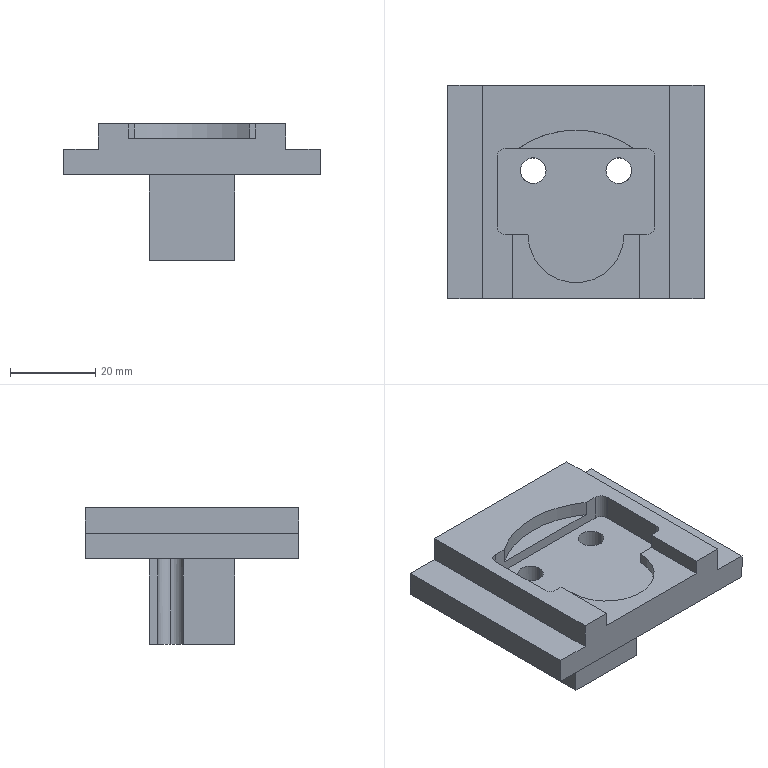Part | SolidWorks | features Cut 4, ICE 4, Extrusion 1, Fillet 1, MirrorPattern 1 | 1 solid | 37 faces | box 60 x 50 x 32 mm | volume 31490 mm3 | plane 27 | cylinder 10 | commonest cylinder face diameters 4 x4 6 x4 22.5 x1 47 x1
STEP:
#1=CARTESIAN_POINT('',(-7.,5.,6.));
#2=VERTEX_POINT('',#1);
#3=CARTESIAN_POINT('',(-13.,5.,6.));
#4=VERTEX_POINT('',#3);
#5=CARTESIAN_POINT('',(-10.,5.,6.));
#6=DIRECTION('',(0.,0.,-1.));
#7=DIRECTION('',(1.,0.,0.));
#8=AXIS2_PLACEMENT_3D('',#5,#6,#7);
#9=CIRCLE('',#8,3.);
#10=EDGE_CURVE('',#2,#4,#9,.T.);
#11=ORIENTED_EDGE('',*,*,#10,.F.);
#12=CARTESIAN_POINT('',(-7.,5.,-20.));
#13=VERTEX_POINT('',#12);
#14=CARTESIAN_POINT('',(-7.,5.,12.));
#15=DIRECTION('',(0.,0.,-1.));
#16=VECTOR('',#15,1000.);
#17=LINE('',#14,#16);
#18=EDGE_CURVE('',#2,#13,#17,.T.);
#19=ORIENTED_EDGE('',*,*,#18,.T.);
#20=CARTESIAN_POINT('',(-10.,2.,-20.));
#21=VERTEX_POINT('',#20);
#22=CARTESIAN_POINT('',(-10.,5.,-20.));
#23=DIRECTION('',(0.,0.,1.));
#24=DIRECTION('',(-1.,0.,0.));
#25=AXIS2_PLACEMENT_3D('',#22,#23,#24);
#26=CIRCLE('',#25,3.);
#27=EDGE_CURVE('',#21,#13,#26,.T.);
#28=ORIENTED_EDGE('',*,*,#27,.F.);
#29=CARTESIAN_POINT('',(-10.,2.,0.));
#30=VERTEX_POINT('',#29);
#31=CARTESIAN_POINT('',(-10.,2.,-20.001));
#32=DIRECTION('',(0.,0.,1.));
#33=VECTOR('',#32,1000.);
#34=LINE('',#31,#33);
#35=EDGE_CURVE('',#21,#30,#34,.T.);
#36=ORIENTED_EDGE('',*,*,#35,.T.);
#37=CARTESIAN_POINT('',(-13.,5.,0.));
#38=VERTEX_POINT('',#37);
#39=CARTESIAN_POINT('',(-10.,5.,0.));
#40=DIRECTION('',(0.,0.,-1.));
#41=DIRECTION('',(1.,0.,0.));
#42=AXIS2_PLACEMENT_3D('',#39,#40,#41);
#43=CIRCLE('',#42,3.);
#44=EDGE_CURVE('',#30,#38,#43,.T.);
#45=ORIENTED_EDGE('',*,*,#44,.T.);
#46=CARTESIAN_POINT('',(-13.,5.,12.));
#47=DIRECTION('',(0.,0.,-1.));
#48=VECTOR('',#47,1000.);
#49=LINE('',#46,#48);
#50=EDGE_CURVE('',#4,#38,#49,.T.);
#51=ORIENTED_EDGE('',*,*,#50,.F.);
#52=EDGE_LOOP('',(#11,#19,#28,#36,#45,#51));
#53=FACE_OUTER_BOUND('',#52,.T.);
#54=CARTESIAN_POINT('',(-10.,5.,12.));
#55=DIRECTION('',(0.,0.,-1.));
#56=DIRECTION('',(-1.,0.,0.));
#57=AXIS2_PLACEMENT_3D('',#54,#55,#56);
#58=CYLINDRICAL_SURFACE('',#57,3.);
#59=ADVANCED_FACE('',(#53),#58,.F.);
#60=CARTESIAN_POINT('',(13.,5.,6.));
#61=VERTEX_POINT('',#60);
#62=CARTESIAN_POINT('',(7.,5.,6.));
#63=VERTEX_POINT('',#62);
#64=CARTESIAN_POINT('',(10.,5.,6.));
#65=DIRECTION('',(0.,0.,-1.));
#66=DIRECTION('',(1.,0.,0.));
#67=AXIS2_PLACEMENT_3D('',#64,#65,#66);
#68=CIRCLE('',#67,3.);
#69=EDGE_CURVE('',#61,#63,#68,.T.);
#70=ORIENTED_EDGE('',*,*,#69,.F.);
#71=CARTESIAN_POINT('',(13.,5.,0.));
#72=VERTEX_POINT('',#71);
#73=CARTESIAN_POINT('',(13.,5.,12.));
#74=DIRECTION('',(0.,0.,-1.));
#75=VECTOR('',#74,1000.);
#76=LINE('',#73,#75);
#77=EDGE_CURVE('',#61,#72,#76,.T.);
#78=ORIENTED_EDGE('',*,*,#77,.T.);
#79=CARTESIAN_POINT('',(10.,2.,0.));
#80=VERTEX_POINT('',#79);
#81=CARTESIAN_POINT('',(10.,5.,0.));
#82=DIRECTION('',(0.,0.,-1.));
#83=DIRECTION('',(1.,0.,0.));
#84=AXIS2_PLACEMENT_3D('',#81,#82,#83);
#85=CIRCLE('',#84,3.);
#86=EDGE_CURVE('',#72,#80,#85,.T.);
#87=ORIENTED_EDGE('',*,*,#86,.T.);
#88=CARTESIAN_POINT('',(10.,2.,-20.));
#89=VERTEX_POINT('',#88);
#90=CARTESIAN_POINT('',(10.,2.,-20.001));
#91=DIRECTION('',(0.,0.,-1.));
#92=VECTOR('',#91,1000.);
#93=LINE('',#90,#92);
#94=EDGE_CURVE('',#80,#89,#93,.T.);
#95=ORIENTED_EDGE('',*,*,#94,.T.);
#96=CARTESIAN_POINT('',(7.,5.,-20.));
#97=VERTEX_POINT('',#96);
#98=CARTESIAN_POINT('',(10.,5.,-20.));
#99=DIRECTION('',(0.,0.,1.));
#100=DIRECTION('',(-1.,0.,0.));
#101=AXIS2_PLACEMENT_3D('',#98,#99,#100);
#102=CIRCLE('',#101,3.);
#103=EDGE_CURVE('',#97,#89,#102,.T.);
#104=ORIENTED_EDGE('',*,*,#103,.F.);
#105=CARTESIAN_POINT('',(7.,5.,12.));
#106=DIRECTION('',(0.,0.,-1.));
#107=VECTOR('',#106,1000.);
#108=LINE('',#105,#107);
#109=EDGE_CURVE('',#63,#97,#108,.T.);
#110=ORIENTED_EDGE('',*,*,#109,.F.);
#111=EDGE_LOOP('',(#70,#78,#87,#95,#104,#110));
#112=FACE_OUTER_BOUND('',#111,.T.);
#113=CARTESIAN_POINT('',(10.,5.,12.));
#114=DIRECTION('',(0.,0.,-1.));
#115=DIRECTION('',(-1.,0.,0.));
#116=AXIS2_PLACEMENT_3D('',#113,#114,#115);
#117=CYLINDRICAL_SURFACE('',#116,3.);
#118=ADVANCED_FACE('',(#112),#117,.F.);
#119=ORIENTED_EDGE('',*,*,#77,.F.);
#120=CARTESIAN_POINT('',(10.,5.,6.));
#121=DIRECTION('',(0.,0.,-1.));
#122=DIRECTION('',(1.,0.,0.));
#123=AXIS2_PLACEMENT_3D('',#120,#121,#122);
#124=CIRCLE('',#123,3.);
#125=EDGE_CURVE('',#63,#61,#124,.T.);
#126=ORIENTED_EDGE('',*,*,#125,.F.);
#127=ORIENTED_EDGE('',*,*,#109,.T.);
#128=CARTESIAN_POINT('',(10.,8.,-20.));
#129=VERTEX_POINT('',#128);
#130=CARTESIAN_POINT('',(10.,5.,-20.));
#131=DIRECTION('',(0.,0.,1.));
#132=DIRECTION('',(-1.,0.,0.));
#133=AXIS2_PLACEMENT_3D('',#130,#131,#132);
#134=CIRCLE('',#133,3.);
#135=EDGE_CURVE('',#129,#97,#134,.T.);
#136=ORIENTED_EDGE('',*,*,#135,.F.);
#137=CARTESIAN_POINT('',(10.,8.,0.));
#138=VERTEX_POINT('',#137);
#139=CARTESIAN_POINT('',(10.,8.,-20.001));
#140=DIRECTION('',(0.,0.,1.));
#141=VECTOR('',#140,1000.);
#142=LINE('',#139,#141);
#143=EDGE_CURVE('',#129,#138,#142,.T.);
#144=ORIENTED_EDGE('',*,*,#143,.T.);
#145=CARTESIAN_POINT('',(10.,5.,0.));
#146=DIRECTION('',(0.,0.,-1.));
#147=DIRECTION('',(1.,0.,0.));
#148=AXIS2_PLACEMENT_3D('',#145,#146,#147);
#149=CIRCLE('',#148,3.);
#150=EDGE_CURVE('',#138,#72,#149,.T.);
#151=ORIENTED_EDGE('',*,*,#150,.T.);
#152=EDGE_LOOP('',(#119,#126,#127,#136,#144,#151));
#153=FACE_OUTER_BOUND('',#152,.T.);
#154=CARTESIAN_POINT('',(10.,5.,12.));
#155=DIRECTION('',(0.,0.,-1.));
#156=DIRECTION('',(-1.,0.,0.));
#157=AXIS2_PLACEMENT_3D('',#154,#155,#156);
#158=CYLINDRICAL_SURFACE('',#157,3.);
#159=ADVANCED_FACE('',(#153),#158,.F.);
#160=CARTESIAN_POINT('',(11.25,-10.,8.5));
#161=VERTEX_POINT('',#160);
#162=CARTESIAN_POINT('',(14.923,-10.,8.5));
#163=VERTEX_POINT('',#162);
#164=CARTESIAN_POINT('',(17.,-10.,8.5));
#165=DIRECTION('',(1.,0.,0.));
#166=VECTOR('',#165,1000.);
#167=LINE('',#164,#166);
#168=EDGE_CURVE('',#161,#163,#167,.T.);
#169=ORIENTED_EDGE('',*,*,#168,.F.);
#170=CARTESIAN_POINT('',(-11.25,-10.,8.5));
#171=VERTEX_POINT('',#170);
#172=CARTESIAN_POINT('',(0.,-10.,8.5));
#173=DIRECTION('',(0.,0.,1.));
#174=DIRECTION('',(1.,0.,0.));
#175=AXIS2_PLACEMENT_3D('',#172,#173,#174);
#176=CIRCLE('',#175,11.25);
#177=EDGE_CURVE('',#171,#161,#176,.T.);
#178=ORIENTED_EDGE('',*,*,#177,.F.);
#179=CARTESIAN_POINT('',(-14.923,-10.,8.5));
#180=VERTEX_POINT('',#179);
#181=CARTESIAN_POINT('',(17.,-10.,8.5));
#182=DIRECTION('',(-1.,0.,0.));
#183=VECTOR('',#182,1000.);
#184=LINE('',#181,#183);
#185=EDGE_CURVE('',#171,#180,#184,.T.);
#186=ORIENTED_EDGE('',*,*,#185,.T.);
#187=CARTESIAN_POINT('',(-14.923,-25.,8.5));
#188=VERTEX_POINT('',#187);
#189=CARTESIAN_POINT('',(-14.923,0.,8.5));
#190=DIRECTION('',(0.,-1.,0.));
#191=VECTOR('',#190,1000.);
#192=LINE('',#189,#191);
#193=EDGE_CURVE('',#180,#188,#192,.T.);
#194=ORIENTED_EDGE('',*,*,#193,.T.);
#195=CARTESIAN_POINT('',(14.923,-25.,8.5));
#196=VERTEX_POINT('',#195);
#197=CARTESIAN_POINT('',(0.,-25.,8.5));
#198=DIRECTION('',(1.,0.,0.));
#199=VECTOR('',#198,1000.);
#200=LINE('',#197,#199);
#201=EDGE_CURVE('',#188,#196,#200,.T.);
#202=ORIENTED_EDGE('',*,*,#201,.T.);
#203=CARTESIAN_POINT('',(14.923,0.,8.5));
#204=DIRECTION('',(0.,-1.,0.));
#205=VECTOR('',#204,1000.);
#206=LINE('',#203,#205);
#207=EDGE_CURVE('',#163,#196,#206,.T.);
#208=ORIENTED_EDGE('',*,*,#207,.F.);
#209=EDGE_LOOP('',(#169,#178,#186,#194,#202,#208));
#210=FACE_OUTER_BOUND('',#209,.T.);
#211=CARTESIAN_POINT('',(17.,4.964,8.5));
#212=DIRECTION('',(0.,0.,1.));
#213=DIRECTION('',(1.,0.,0.));
#214=AXIS2_PLACEMENT_3D('',#211,#212,#213);
#215=PLANE('',#214);
#216=ADVANCED_FACE('',(#210),#215,.T.);
#217=CARTESIAN_POINT('',(14.923,-10.,12.));
#218=VERTEX_POINT('',#217);
#219=CARTESIAN_POINT('',(16.5,-10.,12.));
#220=VERTEX_POINT('',#219);
#221=CARTESIAN_POINT('',(0.,-10.,12.));
#222=DIRECTION('',(1.,0.,0.));
#223=VECTOR('',#222,1000.);
#224=LINE('',#221,#223);
#225=EDGE_CURVE('',#218,#220,#224,.T.);
#226=ORIENTED_EDGE('',*,*,#225,.F.);
#227=CARTESIAN_POINT('',(14.923,-25.,12.));
#228=VERTEX_POINT('',#227);
#229=CARTESIAN_POINT('',(14.923,0.,12.));
#230=DIRECTION('',(0.,-1.,0.));
#231=VECTOR('',#230,1000.);
#232=LINE('',#229,#231);
#233=EDGE_CURVE('',#218,#228,#232,.T.);
#234=ORIENTED_EDGE('',*,*,#233,.T.);
#235=CARTESIAN_POINT('',(22.,-25.,12.));
#236=VERTEX_POINT('',#235);
#237=CARTESIAN_POINT('',(30.,-25.,12.));
#238=DIRECTION('',(1.,0.,0.));
#239=VECTOR('',#238,1000.);
#240=LINE('',#237,#239);
#241=EDGE_CURVE('',#228,#236,#240,.T.);
#242=ORIENTED_EDGE('',*,*,#241,.T.);
#243=CARTESIAN_POINT('',(22.,25.,12.));
#244=VERTEX_POINT('',#243);
#245=CARTESIAN_POINT('',(22.,-25.,12.));
#246=DIRECTION('',(0.,-1.,0.));
#247=VECTOR('',#246,1000.);
#248=LINE('',#245,#247);
#249=EDGE_CURVE('',#244,#236,#248,.T.);
#250=ORIENTED_EDGE('',*,*,#249,.F.);
#251=CARTESIAN_POINT('',(-22.,25.,12.));
#252=VERTEX_POINT('',#251);
#253=CARTESIAN_POINT('',(30.,25.,12.));
#254=DIRECTION('',(-1.,0.,0.));
#255=VECTOR('',#254,1000.);
#256=LINE('',#253,#255);
#257=EDGE_CURVE('',#244,#252,#256,.T.);
#258=ORIENTED_EDGE('',*,*,#257,.T.);
#259=CARTESIAN_POINT('',(-22.,-25.,12.));
#260=VERTEX_POINT('',#259);
#261=CARTESIAN_POINT('',(-22.,25.,12.));
#262=DIRECTION('',(0.,1.,0.));
#263=VECTOR('',#262,1000.);
#264=LINE('',#261,#263);
#265=EDGE_CURVE('',#260,#252,#264,.T.);
#266=ORIENTED_EDGE('',*,*,#265,.F.);
#267=CARTESIAN_POINT('',(-14.923,-25.,12.));
#268=VERTEX_POINT('',#267);
#269=CARTESIAN_POINT('',(30.,-25.,12.));
#270=DIRECTION('',(1.,0.,0.));
#271=VECTOR('',#270,1000.);
#272=LINE('',#269,#271);
#273=EDGE_CURVE('',#260,#268,#272,.T.);
#274=ORIENTED_EDGE('',*,*,#273,.T.);
#275=CARTESIAN_POINT('',(-14.923,-10.,12.));
#276=VERTEX_POINT('',#275);
#277=CARTESIAN_POINT('',(-14.923,0.,12.));
#278=DIRECTION('',(0.,-1.,0.));
#279=VECTOR('',#278,1000.);
#280=LINE('',#277,#279);
#281=EDGE_CURVE('',#276,#268,#280,.T.);
#282=ORIENTED_EDGE('',*,*,#281,.F.);
#283=CARTESIAN_POINT('',(-16.5,-10.,12.));
#284=VERTEX_POINT('',#283);
#285=CARTESIAN_POINT('',(0.,-10.,12.));
#286=DIRECTION('',(-1.,0.,0.));
#287=VECTOR('',#286,1000.);
#288=LINE('',#285,#287);
#289=EDGE_CURVE('',#276,#284,#288,.T.);
#290=ORIENTED_EDGE('',*,*,#289,.T.);
#291=CARTESIAN_POINT('',(-18.5,-8.,12.));
#292=VERTEX_POINT('',#291);
#293=CARTESIAN_POINT('',(-16.5,-8.,12.));
#294=DIRECTION('',(0.,0.,-1.));
#295=DIRECTION('',(1.,0.,0.));
#296=AXIS2_PLACEMENT_3D('',#293,#294,#295);
#297=CIRCLE('',#296,2.);
#298=EDGE_CURVE('',#284,#292,#297,.T.);
#299=ORIENTED_EDGE('',*,*,#298,.T.);
#300=CARTESIAN_POINT('',(-18.5,8.2,12.));
#301=VERTEX_POINT('',#300);
#302=CARTESIAN_POINT('',(-18.5,4.964,12.));
#303=DIRECTION('',(0.,-1.,0.));
#304=VECTOR('',#303,1000.);
#305=LINE('',#302,#304);
#306=EDGE_CURVE('',#301,#292,#305,.T.);
#307=ORIENTED_EDGE('',*,*,#306,.F.);
#308=CARTESIAN_POINT('',(-16.5,10.2,12.));
#309=VERTEX_POINT('',#308);
#310=CARTESIAN_POINT('',(-16.5,8.2,12.));
#311=DIRECTION('',(0.,0.,-1.));
#312=DIRECTION('',(1.,0.,0.));
#313=AXIS2_PLACEMENT_3D('',#310,#311,#312);
#314=CIRCLE('',#313,2.);
#315=EDGE_CURVE('',#301,#309,#314,.T.);
#316=ORIENTED_EDGE('',*,*,#315,.T.);
#317=CARTESIAN_POINT('',(-13.55,10.2,12.));
#318=VERTEX_POINT('',#317);
#319=CARTESIAN_POINT('',(0.,10.2,12.));
#320=DIRECTION('',(1.,0.,0.));
#321=VECTOR('',#320,1000.);
#322=LINE('',#319,#321);
#323=EDGE_CURVE('',#309,#318,#322,.T.);
#324=ORIENTED_EDGE('',*,*,#323,.T.);
#325=CARTESIAN_POINT('',(13.55,10.2,12.));
#326=VERTEX_POINT('',#325);
#327=CARTESIAN_POINT('',(0.,-9.,12.));
#328=DIRECTION('',(0.,0.,1.));
#329=DIRECTION('',(1.,0.,0.));
#330=AXIS2_PLACEMENT_3D('',#327,#328,#329);
#331=CIRCLE('',#330,23.5);
#332=EDGE_CURVE('',#326,#318,#331,.T.);
#333=ORIENTED_EDGE('',*,*,#332,.F.);
#334=CARTESIAN_POINT('',(16.5,10.2,12.));
#335=VERTEX_POINT('',#334);
#336=CARTESIAN_POINT('',(0.,10.2,12.));
#337=DIRECTION('',(-1.,0.,0.));
#338=VECTOR('',#337,1000.);
#339=LINE('',#336,#338);
#340=EDGE_CURVE('',#335,#326,#339,.T.);
#341=ORIENTED_EDGE('',*,*,#340,.F.);
#342=CARTESIAN_POINT('',(18.5,8.2,12.));
#343=VERTEX_POINT('',#342);
#344=CARTESIAN_POINT('',(16.5,8.2,12.));
#345=DIRECTION('',(0.,0.,-1.));
#346=DIRECTION('',(1.,0.,0.));
#347=AXIS2_PLACEMENT_3D('',#344,#345,#346);
#348=CIRCLE('',#347,2.);
#349=EDGE_CURVE('',#335,#343,#348,.T.);
#350=ORIENTED_EDGE('',*,*,#349,.T.);
#351=CARTESIAN_POINT('',(18.5,-8.,12.));
#352=VERTEX_POINT('',#351);
#353=CARTESIAN_POINT('',(18.5,-1.5,12.));
#354=DIRECTION('',(0.,1.,0.));
#355=VECTOR('',#354,1000.);
#356=LINE('',#353,#355);
#357=EDGE_CURVE('',#352,#343,#356,.T.);
#358=ORIENTED_EDGE('',*,*,#357,.F.);
#359=CARTESIAN_POINT('',(16.5,-8.,12.));
#360=DIRECTION('',(0.,0.,-1.));
#361=DIRECTION('',(1.,0.,0.));
#362=AXIS2_PLACEMENT_3D('',#359,#360,#361);
#363=CIRCLE('',#362,2.);
#364=EDGE_CURVE('',#352,#220,#363,.T.);
#365=ORIENTED_EDGE('',*,*,#364,.T.);
#366=EDGE_LOOP('',(#226,#234,#242,#250,#258,#266,#274,#282,#290,#299,#307,#316,#324,#333,#341,#350,#358,#365));
#367=FACE_OUTER_BOUND('',#366,.T.);
#368=CARTESIAN_POINT('',(0.,0.,12.));
#369=DIRECTION('',(0.,0.,1.));
#370=DIRECTION('',(1.,0.,0.));
#371=AXIS2_PLACEMENT_3D('',#368,#369,#370);
#372=PLANE('',#371);
#373=ADVANCED_FACE('',(#367),#372,.T.);
#374=CARTESIAN_POINT('',(13.55,10.2,8.5));
#375=VERTEX_POINT('',#374);
#376=CARTESIAN_POINT('',(-13.55,10.2,8.5));
#377=VERTEX_POINT('',#376);
#378=CARTESIAN_POINT('',(0.,-9.,8.5));
#379=DIRECTION('',(0.,0.,1.));
#380=DIRECTION('',(1.,0.,0.));
#381=AXIS2_PLACEMENT_3D('',#378,#379,#380);
#382=CIRCLE('',#381,23.5);
#383=EDGE_CURVE('',#375,#377,#382,.T.);
#384=ORIENTED_EDGE('',*,*,#383,.F.);
#385=CARTESIAN_POINT('',(13.55,10.2,8.5));
#386=DIRECTION('',(0.,0.,1.));
#387=VECTOR('',#386,1000.);
#388=LINE('',#385,#387);
#389=EDGE_CURVE('',#375,#326,#388,.T.);
#390=ORIENTED_EDGE('',*,*,#389,.T.);
#391=ORIENTED_EDGE('',*,*,#332,.T.);
#392=CARTESIAN_POINT('',(-13.55,10.2,8.5));
#393=DIRECTION('',(0.,0.,1.));
#394=VECTOR('',#393,1000.);
#395=LINE('',#392,#394);
#396=EDGE_CURVE('',#377,#318,#395,.T.);
#397=ORIENTED_EDGE('',*,*,#396,.F.);
#398=EDGE_LOOP('',(#384,#390,#391,#397));
#399=FACE_OUTER_BOUND('',#398,.T.);
#400=CARTESIAN_POINT('',(0.,-9.,8.5));
#401=DIRECTION('',(0.,0.,1.));
#402=DIRECTION('',(1.,0.,0.));
#403=AXIS2_PLACEMENT_3D('',#400,#401,#402);
#404=CYLINDRICAL_SURFACE('',#403,23.5);
#405=ADVANCED_FACE('',(#399),#404,.F.);
#406=CARTESIAN_POINT('',(3.937,10.2,8.5));
#407=DIRECTION('',(-1.,0.,0.));
#408=VECTOR('',#407,1000.);
#409=LINE('',#406,#408);
#410=EDGE_CURVE('',#375,#377,#409,.T.);
#411=ORIENTED_EDGE('',*,*,#410,.F.);
#412=ORIENTED_EDGE('',*,*,#383,.T.);
#413=EDGE_LOOP('',(#411,#412));
#414=FACE_OUTER_BOUND('',#413,.T.);
#415=CARTESIAN_POINT('',(17.,4.964,8.5));
#416=DIRECTION('',(0.,0.,1.));
#417=DIRECTION('',(1.,0.,0.));
#418=AXIS2_PLACEMENT_3D('',#415,#416,#417);
#419=PLANE('',#418);
#420=ADVANCED_FACE('',(#414),#419,.T.);
#421=CARTESIAN_POINT('',(-14.923,-10.,8.5));
#422=DIRECTION('',(0.,0.,-1.));
#423=VECTOR('',#422,1000.);
#424=LINE('',#421,#423);
#425=EDGE_CURVE('',#276,#180,#424,.T.);
#426=ORIENTED_EDGE('',*,*,#425,.F.);
#427=ORIENTED_EDGE('',*,*,#281,.T.);
#428=CARTESIAN_POINT('',(-14.923,-25.,8.5));
#429=DIRECTION('',(0.,0.,1.));
#430=VECTOR('',#429,1000.);
#431=LINE('',#428,#430);
#432=EDGE_CURVE('',#188,#268,#431,.T.);
#433=ORIENTED_EDGE('',*,*,#432,.F.);
#434=ORIENTED_EDGE('',*,*,#193,.F.);
#435=EDGE_LOOP('',(#426,#427,#433,#434));
#436=FACE_OUTER_BOUND('',#435,.T.);
#437=CARTESIAN_POINT('',(-14.923,0.,8.5));
#438=DIRECTION('',(-1.,0.,0.));
#439=DIRECTION('',(0.,0.,1.));
#440=AXIS2_PLACEMENT_3D('',#437,#438,#439);
#441=PLANE('',#440);
#442=ADVANCED_FACE('',(#436),#441,.F.);
#443=ORIENTED_EDGE('',*,*,#177,.T.);
#444=CARTESIAN_POINT('',(11.25,-10.,6.));
#445=VERTEX_POINT('',#444);
#446=CARTESIAN_POINT('',(11.25,-10.,6.));
#447=DIRECTION('',(0.,0.,-1.));
#448=VECTOR('',#447,1000.);
#449=LINE('',#446,#448);
#450=EDGE_CURVE('',#161,#445,#449,.T.);
#451=ORIENTED_EDGE('',*,*,#450,.T.);
#452=CARTESIAN_POINT('',(-11.25,-10.,6.));
#453=VERTEX_POINT('',#452);
#454=CARTESIAN_POINT('',(0.,-10.,6.));
#455=DIRECTION('',(0.,0.,1.));
#456=DIRECTION('',(1.,0.,0.));
#457=AXIS2_PLACEMENT_3D('',#454,#455,#456);
#458=CIRCLE('',#457,11.25);
#459=EDGE_CURVE('',#453,#445,#458,.T.);
#460=ORIENTED_EDGE('',*,*,#459,.F.);
#461=CARTESIAN_POINT('',(-11.25,-10.,6.));
#462=DIRECTION('',(0.,0.,-1.));
#463=VECTOR('',#462,1000.);
#464=LINE('',#461,#463);
#465=EDGE_CURVE('',#171,#453,#464,.T.);
#466=ORIENTED_EDGE('',*,*,#465,.F.);
#467=EDGE_LOOP('',(#443,#451,#460,#466));
#468=FACE_OUTER_BOUND('',#467,.T.);
#469=CARTESIAN_POINT('',(0.,-10.,6.));
#470=DIRECTION('',(0.,0.,1.));
#471=DIRECTION('',(1.,0.,0.));
#472=AXIS2_PLACEMENT_3D('',#469,#470,#471);
#473=CYLINDRICAL_SURFACE('',#472,11.25);
#474=ADVANCED_FACE('',(#468),#473,.F.);
#475=ORIENTED_EDGE('',*,*,#18,.F.);
#476=CARTESIAN_POINT('',(-10.,5.,6.));
#477=DIRECTION('',(0.,0.,-1.));
#478=DIRECTION('',(1.,0.,0.));
#479=AXIS2_PLACEMENT_3D('',#476,#477,#478);
#480=CIRCLE('',#479,3.);
#481=EDGE_CURVE('',#4,#2,#480,.T.);
#482=ORIENTED_EDGE('',*,*,#481,.F.);
#483=ORIENTED_EDGE('',*,*,#50,.T.);
#484=CARTESIAN_POINT('',(-10.,8.,0.));
#485=VERTEX_POINT('',#484);
#486=CARTESIAN_POINT('',(-10.,5.,0.));
#487=DIRECTION('',(0.,0.,-1.));
#488=DIRECTION('',(1.,0.,0.));
#489=AXIS2_PLACEMENT_3D('',#486,#487,#488);
#490=CIRCLE('',#489,3.);
#491=EDGE_CURVE('',#38,#485,#490,.T.);
#492=ORIENTED_EDGE('',*,*,#491,.T.);
#493=CARTESIAN_POINT('',(-10.,8.,-20.));
#494=VERTEX_POINT('',#493);
#495=CARTESIAN_POINT('',(-10.,8.,-20.001));
#496=DIRECTION('',(0.,0.,-1.));
#497=VECTOR('',#496,1000.);
#498=LINE('',#495,#497);
#499=EDGE_CURVE('',#485,#494,#498,.T.);
#500=ORIENTED_EDGE('',*,*,#499,.T.);
#501=CARTESIAN_POINT('',(-10.,5.,-20.));
#502=DIRECTION('',(0.,0.,1.));
#503=DIRECTION('',(-1.,0.,0.));
#504=AXIS2_PLACEMENT_3D('',#501,#502,#503);
#505=CIRCLE('',#504,3.);
#506=EDGE_CURVE('',#13,#494,#505,.T.);
#507=ORIENTED_EDGE('',*,*,#506,.F.);
#508=EDGE_LOOP('',(#475,#482,#483,#492,#500,#507));
#509=FACE_OUTER_BOUND('',#508,.T.);
#510=CARTESIAN_POINT('',(-10.,5.,12.));
#511=DIRECTION('',(0.,0.,-1.));
#512=DIRECTION('',(-1.,0.,0.));
#513=AXIS2_PLACEMENT_3D('',#510,#511,#512);
#514=CYLINDRICAL_SURFACE('',#513,3.);
#515=ADVANCED_FACE('',(#509),#514,.F.);
#516=CARTESIAN_POINT('',(-30.,25.,6.));
#517=VERTEX_POINT('',#516);
#518=CARTESIAN_POINT('',(-30.,-25.,6.));
#519=VERTEX_POINT('',#518);
#520=CARTESIAN_POINT('',(-30.,25.,6.));
#521=DIRECTION('',(0.,-1.,0.));
#522=VECTOR('',#521,1000.);
#523=LINE('',#520,#522);
#524=EDGE_CURVE('',#517,#519,#523,.T.);
#525=ORIENTED_EDGE('',*,*,#524,.F.);
#526=CARTESIAN_POINT('',(-30.,25.,0.));
#527=VERTEX_POINT('',#526);
#528=CARTESIAN_POINT('',(-30.,25.,12.));
#529=DIRECTION('',(0.,0.,-1.));
#530=VECTOR('',#529,1000.);
#531=LINE('',#528,#530);
#532=EDGE_CURVE('',#517,#527,#531,.T.);
#533=ORIENTED_EDGE('',*,*,#532,.T.);
#534=CARTESIAN_POINT('',(-30.,-25.,0.));
#535=VERTEX_POINT('',#534);
#536=CARTESIAN_POINT('',(-30.,-25.,0.));
#537=DIRECTION('',(0.,-1.,0.));
#538=VECTOR('',#537,1000.);
#539=LINE('',#536,#538);
#540=EDGE_CURVE('',#527,#535,#539,.T.);
#541=ORIENTED_EDGE('',*,*,#540,.T.);
#542=CARTESIAN_POINT('',(-30.,-25.,12.));
#543=DIRECTION('',(0.,0.,-1.));
#544=VECTOR('',#543,1000.);
#545=LINE('',#542,#544);
#546=EDGE_CURVE('',#519,#535,#545,.T.);
#547=ORIENTED_EDGE('',*,*,#546,.F.);
#548=EDGE_LOOP('',(#525,#533,#541,#547));
#549=FACE_OUTER_BOUND('',#548,.T.);
#550=CARTESIAN_POINT('',(-30.,-25.,12.));
#551=DIRECTION('',(1.,0.,0.));
#552=DIRECTION('',(0.,0.,-1.));
#553=AXIS2_PLACEMENT_3D('',#550,#551,#552);
#554=PLANE('',#553);
#555=ADVANCED_FACE('',(#549),#554,.F.);
#556=CARTESIAN_POINT('',(30.,-25.,6.));
#557=VERTEX_POINT('',#556);
#558=CARTESIAN_POINT('',(30.,25.,6.));
#559=VERTEX_POINT('',#558);
#560=CARTESIAN_POINT('',(30.,-25.,6.));
#561=DIRECTION('',(0.,1.,0.));
#562=VECTOR('',#561,1000.);
#563=LINE('',#560,#562);
#564=EDGE_CURVE('',#557,#559,#563,.T.);
#565=ORIENTED_EDGE('',*,*,#564,.F.);
#566=CARTESIAN_POINT('',(30.,-25.,0.));
#567=VERTEX_POINT('',#566);
#568=CARTESIAN_POINT('',(30.,-25.,12.));
#569=DIRECTION('',(0.,0.,-1.));
#570=VECTOR('',#569,1000.);
#571=LINE('',#568,#570);
#572=EDGE_CURVE('',#557,#567,#571,.T.);
#573=ORIENTED_EDGE('',*,*,#572,.T.);
#574=CARTESIAN_POINT('',(30.,25.,0.));
#575=VERTEX_POINT('',#574);
#576=CARTESIAN_POINT('',(30.,-25.,0.));
#577=DIRECTION('',(0.,1.,0.));
#578=VECTOR('',#577,1000.);
#579=LINE('',#576,#578);
#580=EDGE_CURVE('',#567,#575,#579,.T.);
#581=ORIENTED_EDGE('',*,*,#580,.T.);
#582=CARTESIAN_POINT('',(30.,25.,12.));
#583=DIRECTION('',(0.,0.,-1.));
#584=VECTOR('',#583,1000.);
#585=LINE('',#582,#584);
#586=EDGE_CURVE('',#559,#575,#585,.T.);
#587=ORIENTED_EDGE('',*,*,#586,.F.);
#588=EDGE_LOOP('',(#565,#573,#581,#587));
#589=FACE_OUTER_BOUND('',#588,.T.);
#590=CARTESIAN_POINT('',(30.,-25.,12.));
#591=DIRECTION('',(-1.,0.,0.));
#592=DIRECTION('',(0.,-1.,0.));
#593=AXIS2_PLACEMENT_3D('',#590,#591,#592);
#594=PLANE('',#593);
#595=ADVANCED_FACE('',(#589),#594,.F.);
#596=ORIENTED_EDGE('',*,*,#540,.F.);
#597=CARTESIAN_POINT('',(30.,25.,0.));
#598=DIRECTION('',(-1.,0.,0.));
#599=VECTOR('',#598,1000.);
#600=LINE('',#597,#599);
#601=EDGE_CURVE('',#575,#527,#600,.T.);
#602=ORIENTED_EDGE('',*,*,#601,.F.);
#603=ORIENTED_EDGE('',*,*,#580,.F.);
#604=CARTESIAN_POINT('',(30.,-25.,0.));
#605=DIRECTION('',(1.,0.,0.));
#606=VECTOR('',#605,1000.);
#607=LINE('',#604,#606);
#608=EDGE_CURVE('',#535,#567,#607,.T.);
#609=ORIENTED_EDGE('',*,*,#608,.F.);
#610=EDGE_LOOP('',(#596,#602,#603,#609));
#611=FACE_OUTER_BOUND('',#610,.T.);
#612=ORIENTED_EDGE('',*,*,#44,.F.);
#613=CARTESIAN_POINT('',(-10.,-10.,0.));
#614=VERTEX_POINT('',#613);
#615=CARTESIAN_POINT('',(-10.,-10.,0.));
#616=DIRECTION('',(0.,1.,0.));
#617=VECTOR('',#616,1000.);
#618=LINE('',#615,#617);
#619=EDGE_CURVE('',#614,#30,#618,.T.);
#620=ORIENTED_EDGE('',*,*,#619,.F.);
#621=CARTESIAN_POINT('',(10.,-10.,0.));
#622=VERTEX_POINT('',#621);
#623=CARTESIAN_POINT('',(-10.,-10.,0.));
#624=DIRECTION('',(-1.,0.,0.));
#625=VECTOR('',#624,1000.);
#626=LINE('',#623,#625);
#627=EDGE_CURVE('',#622,#614,#626,.T.);
#628=ORIENTED_EDGE('',*,*,#627,.F.);
#629=CARTESIAN_POINT('',(10.,-10.,0.));
#630=DIRECTION('',(0.,-1.,0.));
#631=VECTOR('',#630,1000.);
#632=LINE('',#629,#631);
#633=EDGE_CURVE('',#80,#622,#632,.T.);
#634=ORIENTED_EDGE('',*,*,#633,.F.);
#635=ORIENTED_EDGE('',*,*,#86,.F.);
#636=ORIENTED_EDGE('',*,*,#150,.F.);
#637=CARTESIAN_POINT('',(10.,10.,0.));
#638=VERTEX_POINT('',#637);
#639=CARTESIAN_POINT('',(10.,-10.,0.));
#640=DIRECTION('',(0.,-1.,0.));
#641=VECTOR('',#640,1000.);
#642=LINE('',#639,#641);
#643=EDGE_CURVE('',#638,#138,#642,.T.);
#644=ORIENTED_EDGE('',*,*,#643,.F.);
#645=CARTESIAN_POINT('',(-10.,10.,0.));
#646=VERTEX_POINT('',#645);
#647=CARTESIAN_POINT('',(-10.,10.,0.));
#648=DIRECTION('',(1.,0.,0.));
#649=VECTOR('',#648,1000.);
#650=LINE('',#647,#649);
#651=EDGE_CURVE('',#646,#638,#650,.T.);
#652=ORIENTED_EDGE('',*,*,#651,.F.);
#653=CARTESIAN_POINT('',(-10.,-10.,0.));
#654=DIRECTION('',(0.,1.,0.));
#655=VECTOR('',#654,1000.);
#656=LINE('',#653,#655);
#657=EDGE_CURVE('',#485,#646,#656,.T.);
#658=ORIENTED_EDGE('',*,*,#657,.F.);
#659=ORIENTED_EDGE('',*,*,#491,.F.);
#660=EDGE_LOOP('',(#612,#620,#628,#634,#635,#636,#644,#652,#658,#659));
#661=FACE_BOUND('',#660,.T.);
#662=CARTESIAN_POINT('',(0.,0.,0.));
#663=DIRECTION('',(0.,0.,1.));
#664=DIRECTION('',(1.,0.,0.));
#665=AXIS2_PLACEMENT_3D('',#662,#663,#664);
#666=PLANE('',#665);
#667=ADVANCED_FACE('',(#611,#661),#666,.F.);
#668=ORIENTED_EDGE('',*,*,#143,.F.);
#669=CARTESIAN_POINT('',(10.,10.,-20.));
#670=VERTEX_POINT('',#669);
#671=CARTESIAN_POINT('',(10.,-10.,-20.));
#672=DIRECTION('',(0.,-1.,0.));
#673=VECTOR('',#672,1000.);
#674=LINE('',#671,#673);
#675=EDGE_CURVE('',#670,#129,#674,.T.);
#676=ORIENTED_EDGE('',*,*,#675,.F.);
#677=CARTESIAN_POINT('',(10.,10.,-20.));
#678=DIRECTION('',(0.,0.,1.));
#679=VECTOR('',#678,1000.);
#680=LINE('',#677,#679);
#681=EDGE_CURVE('',#670,#638,#680,.T.);
#682=ORIENTED_EDGE('',*,*,#681,.T.);
#683=ORIENTED_EDGE('',*,*,#643,.T.);
#684=EDGE_LOOP('',(#668,#676,#682,#683));
#685=FACE_OUTER_BOUND('',#684,.T.);
#686=CARTESIAN_POINT('',(10.,-10.,-20.));
#687=DIRECTION('',(-1.,0.,0.));
#688=DIRECTION('',(0.,0.,1.));
#689=AXIS2_PLACEMENT_3D('',#686,#687,#688);
#690=PLANE('',#689);
#691=ADVANCED_FACE('',(#685),#690,.F.);
#692=ORIENTED_EDGE('',*,*,#94,.F.);
#693=ORIENTED_EDGE('',*,*,#633,.T.);
#694=CARTESIAN_POINT('',(10.,-10.,-20.));
#695=VERTEX_POINT('',#694);
#696=CARTESIAN_POINT('',(10.,-10.,-20.));
#697=DIRECTION('',(0.,0.,1.));
#698=VECTOR('',#697,1000.);
#699=LINE('',#696,#698);
#700=EDGE_CURVE('',#695,#622,#699,.T.);
#701=ORIENTED_EDGE('',*,*,#700,.F.);
#702=CARTESIAN_POINT('',(10.,-10.,-20.));
#703=DIRECTION('',(0.,-1.,0.));
#704=VECTOR('',#703,1000.);
#705=LINE('',#702,#704);
#706=EDGE_CURVE('',#89,#695,#705,.T.);
#707=ORIENTED_EDGE('',*,*,#706,.F.);
#708=EDGE_LOOP('',(#692,#693,#701,#707));
#709=FACE_OUTER_BOUND('',#708,.T.);
#710=CARTESIAN_POINT('',(10.,-10.,-20.));
#711=DIRECTION('',(-1.,0.,0.));
#712=DIRECTION('',(0.,0.,1.));
#713=AXIS2_PLACEMENT_3D('',#710,#711,#712);
#714=PLANE('',#713);
#715=ADVANCED_FACE('',(#709),#714,.F.);
#716=ORIENTED_EDGE('',*,*,#35,.F.);
#717=CARTESIAN_POINT('',(-10.,-10.,-20.));
#718=VERTEX_POINT('',#717);
#719=CARTESIAN_POINT('',(-10.,-10.,-20.));
#720=DIRECTION('',(0.,1.,0.));
#721=VECTOR('',#720,1000.);
#722=LINE('',#719,#721);
#723=EDGE_CURVE('',#718,#21,#722,.T.);
#724=ORIENTED_EDGE('',*,*,#723,.F.);
#725=CARTESIAN_POINT('',(-10.,-10.,-20.));
#726=DIRECTION('',(0.,0.,1.));
#727=VECTOR('',#726,1000.);
#728=LINE('',#725,#727);
#729=EDGE_CURVE('',#718,#614,#728,.T.);
#730=ORIENTED_EDGE('',*,*,#729,.T.);
#731=ORIENTED_EDGE('',*,*,#619,.T.);
#732=EDGE_LOOP('',(#716,#724,#730,#731));
#733=FACE_OUTER_BOUND('',#732,.T.);
#734=CARTESIAN_POINT('',(-10.,-10.,-20.));
#735=DIRECTION('',(1.,0.,0.));
#736=DIRECTION('',(0.,0.,-1.));
#737=AXIS2_PLACEMENT_3D('',#734,#735,#736);
#738=PLANE('',#737);
#739=ADVANCED_FACE('',(#733),#738,.F.);
#740=ORIENTED_EDGE('',*,*,#499,.F.);
#741=ORIENTED_EDGE('',*,*,#657,.T.);
#742=CARTESIAN_POINT('',(-10.,10.,-20.));
#743=VERTEX_POINT('',#742);
#744=CARTESIAN_POINT('',(-10.,10.,-20.));
#745=DIRECTION('',(0.,0.,1.));
#746=VECTOR('',#745,1000.);
#747=LINE('',#744,#746);
#748=EDGE_CURVE('',#743,#646,#747,.T.);
#749=ORIENTED_EDGE('',*,*,#748,.F.);
#750=CARTESIAN_POINT('',(-10.,-10.,-20.));
#751=DIRECTION('',(0.,1.,0.));
#752=VECTOR('',#751,1000.);
#753=LINE('',#750,#752);
#754=EDGE_CURVE('',#494,#743,#753,.T.);
#755=ORIENTED_EDGE('',*,*,#754,.F.);
#756=EDGE_LOOP('',(#740,#741,#749,#755));
#757=FACE_OUTER_BOUND('',#756,.T.);
#758=CARTESIAN_POINT('',(-10.,-10.,-20.));
#759=DIRECTION('',(1.,0.,0.));
#760=DIRECTION('',(0.,0.,-1.));
#761=AXIS2_PLACEMENT_3D('',#758,#759,#760);
#762=PLANE('',#761);
#763=ADVANCED_FACE('',(#757),#762,.F.);
#764=ORIENTED_EDGE('',*,*,#723,.T.);
#765=ORIENTED_EDGE('',*,*,#27,.T.);
#766=ORIENTED_EDGE('',*,*,#506,.T.);
#767=ORIENTED_EDGE('',*,*,#754,.T.);
#768=CARTESIAN_POINT('',(-10.,10.,-20.));
#769=DIRECTION('',(1.,0.,0.));
#770=VECTOR('',#769,1000.);
#771=LINE('',#768,#770);
#772=EDGE_CURVE('',#743,#670,#771,.T.);
#773=ORIENTED_EDGE('',*,*,#772,.T.);
#774=ORIENTED_EDGE('',*,*,#675,.T.);
#775=ORIENTED_EDGE('',*,*,#135,.T.);
#776=ORIENTED_EDGE('',*,*,#103,.T.);
#777=ORIENTED_EDGE('',*,*,#706,.T.);
#778=CARTESIAN_POINT('',(-10.,-10.,-20.));
#779=DIRECTION('',(-1.,0.,0.));
#780=VECTOR('',#779,1000.);
#781=LINE('',#778,#780);
#782=EDGE_CURVE('',#695,#718,#781,.T.);
#783=ORIENTED_EDGE('',*,*,#782,.T.);
#784=EDGE_LOOP('',(#764,#765,#766,#767,#773,#774,#775,#776,#777,#783));
#785=FACE_OUTER_BOUND('',#784,.T.);
#786=CARTESIAN_POINT('',(0.,0.,-20.));
#787=DIRECTION('',(0.,0.,-1.));
#788=DIRECTION('',(-1.,0.,0.));
#789=AXIS2_PLACEMENT_3D('',#786,#787,#788);
#790=PLANE('',#789);
#791=ADVANCED_FACE('',(#785),#790,.T.);
#792=ORIENTED_EDGE('',*,*,#273,.F.);
#793=CARTESIAN_POINT('',(-22.,-25.,6.));
#794=VERTEX_POINT('',#793);
#795=CARTESIAN_POINT('',(-22.,-25.,6.));
#796=DIRECTION('',(0.,0.,1.));
#797=VECTOR('',#796,1000.);
#798=LINE('',#795,#797);
#799=EDGE_CURVE('',#794,#260,#798,.T.);
#800=ORIENTED_EDGE('',*,*,#799,.F.);
#801=CARTESIAN_POINT('',(-30.,-25.,6.));
#802=DIRECTION('',(1.,0.,0.));
#803=VECTOR('',#802,1000.);
#804=LINE('',#801,#803);
#805=EDGE_CURVE('',#519,#794,#804,.T.);
#806=ORIENTED_EDGE('',*,*,#805,.F.);
#807=ORIENTED_EDGE('',*,*,#546,.T.);
#808=ORIENTED_EDGE('',*,*,#608,.T.);
#809=ORIENTED_EDGE('',*,*,#572,.F.);
#810=CARTESIAN_POINT('',(22.,-25.,6.));
#811=VERTEX_POINT('',#810);
#812=CARTESIAN_POINT('',(30.,-25.,6.));
#813=DIRECTION('',(1.,0.,0.));
#814=VECTOR('',#813,1000.);
#815=LINE('',#812,#814);
#816=EDGE_CURVE('',#811,#557,#815,.T.);
#817=ORIENTED_EDGE('',*,*,#816,.F.);
#818=CARTESIAN_POINT('',(22.,-25.,6.));
#819=DIRECTION('',(0.,0.,1.));
#820=VECTOR('',#819,1000.);
#821=LINE('',#818,#820);
#822=EDGE_CURVE('',#811,#236,#821,.T.);
#823=ORIENTED_EDGE('',*,*,#822,.T.);
#824=ORIENTED_EDGE('',*,*,#241,.F.);
#825=CARTESIAN_POINT('',(14.923,-25.,8.5));
#826=DIRECTION('',(0.,0.,1.));
#827=VECTOR('',#826,1000.);
#828=LINE('',#825,#827);
#829=EDGE_CURVE('',#196,#228,#828,.T.);
#830=ORIENTED_EDGE('',*,*,#829,.F.);
#831=ORIENTED_EDGE('',*,*,#201,.F.);
#832=ORIENTED_EDGE('',*,*,#432,.T.);
#833=EDGE_LOOP('',(#792,#800,#806,#807,#808,#809,#817,#823,#824,#830,#831,#832));
#834=FACE_OUTER_BOUND('',#833,.T.);
#835=CARTESIAN_POINT('',(30.,-25.,12.));
#836=DIRECTION('',(0.,1.,0.));
#837=DIRECTION('',(-1.,0.,0.));
#838=AXIS2_PLACEMENT_3D('',#835,#836,#837);
#839=PLANE('',#838);
#840=ADVANCED_FACE('',(#834),#839,.F.);
#841=CARTESIAN_POINT('',(-22.,25.,6.));
#842=VERTEX_POINT('',#841);
#843=CARTESIAN_POINT('',(-30.,25.,6.));
#844=DIRECTION('',(-1.,0.,0.));
#845=VECTOR('',#844,1000.);
#846=LINE('',#843,#845);
#847=EDGE_CURVE('',#842,#517,#846,.T.);
#848=ORIENTED_EDGE('',*,*,#847,.F.);
#849=CARTESIAN_POINT('',(-22.,25.,6.));
#850=DIRECTION('',(0.,0.,1.));
#851=VECTOR('',#850,1000.);
#852=LINE('',#849,#851);
#853=EDGE_CURVE('',#842,#252,#852,.T.);
#854=ORIENTED_EDGE('',*,*,#853,.T.);
#855=ORIENTED_EDGE('',*,*,#257,.F.);
#856=CARTESIAN_POINT('',(22.,25.,6.));
#857=VERTEX_POINT('',#856);
#858=CARTESIAN_POINT('',(22.,25.,6.));
#859=DIRECTION('',(0.,0.,1.));
#860=VECTOR('',#859,1000.);
#861=LINE('',#858,#860);
#862=EDGE_CURVE('',#857,#244,#861,.T.);
#863=ORIENTED_EDGE('',*,*,#862,.F.);
#864=CARTESIAN_POINT('',(30.,25.,6.));
#865=DIRECTION('',(-1.,0.,0.));
#866=VECTOR('',#865,1000.);
#867=LINE('',#864,#866);
#868=EDGE_CURVE('',#559,#857,#867,.T.);
#869=ORIENTED_EDGE('',*,*,#868,.F.);
#870=ORIENTED_EDGE('',*,*,#586,.T.);
#871=ORIENTED_EDGE('',*,*,#601,.T.);
#872=ORIENTED_EDGE('',*,*,#532,.F.);
#873=EDGE_LOOP('',(#848,#854,#855,#863,#869,#870,#871,#872));
#874=FACE_OUTER_BOUND('',#873,.T.);
#875=CARTESIAN_POINT('',(30.,25.,12.));
#876=DIRECTION('',(0.,-1.,0.));
#877=DIRECTION('',(1.,0.,0.));
#878=AXIS2_PLACEMENT_3D('',#875,#876,#877);
#879=PLANE('',#878);
#880=ADVANCED_FACE('',(#874),#879,.F.);
#881=ORIENTED_EDGE('',*,*,#627,.T.);
#882=ORIENTED_EDGE('',*,*,#729,.F.);
#883=ORIENTED_EDGE('',*,*,#782,.F.);
#884=ORIENTED_EDGE('',*,*,#700,.T.);
#885=EDGE_LOOP('',(#881,#882,#883,#884));
#886=FACE_OUTER_BOUND('',#885,.T.);
#887=CARTESIAN_POINT('',(-10.,-10.,-20.));
#888=DIRECTION('',(0.,1.,0.));
#889=DIRECTION('',(-1.,0.,0.));
#890=AXIS2_PLACEMENT_3D('',#887,#888,#889);
#891=PLANE('',#890);
#892=ADVANCED_FACE('',(#886),#891,.F.);
#893=ORIENTED_EDGE('',*,*,#651,.T.);
#894=ORIENTED_EDGE('',*,*,#681,.F.);
#895=ORIENTED_EDGE('',*,*,#772,.F.);
#896=ORIENTED_EDGE('',*,*,#748,.T.);
#897=EDGE_LOOP('',(#893,#894,#895,#896));
#898=FACE_OUTER_BOUND('',#897,.T.);
#899=CARTESIAN_POINT('',(-10.,10.,-20.));
#900=DIRECTION('',(0.,-1.,0.));
#901=DIRECTION('',(1.,0.,0.));
#902=AXIS2_PLACEMENT_3D('',#899,#900,#901);
#903=PLANE('',#902);
#904=ADVANCED_FACE('',(#898),#903,.F.);
#905=CARTESIAN_POINT('',(18.5,-8.,6.));
#906=VERTEX_POINT('',#905);
#907=CARTESIAN_POINT('',(18.5,8.2,6.));
#908=VERTEX_POINT('',#907);
#909=CARTESIAN_POINT('',(18.5,0.,6.));
#910=DIRECTION('',(0.,1.,0.));
#911=VECTOR('',#910,1000.);
#912=LINE('',#909,#911);
#913=EDGE_CURVE('',#906,#908,#912,.T.);
#914=ORIENTED_EDGE('',*,*,#913,.F.);
#915=CARTESIAN_POINT('',(18.5,-8.,12.));
#916=DIRECTION('',(0.,0.,1.));
#917=VECTOR('',#916,1000.);
#918=LINE('',#915,#917);
#919=EDGE_CURVE('',#906,#352,#918,.T.);
#920=ORIENTED_EDGE('',*,*,#919,.T.);
#921=ORIENTED_EDGE('',*,*,#357,.T.);
#922=CARTESIAN_POINT('',(18.5,8.2,6.));
#923=DIRECTION('',(0.,0.,-1.));
#924=VECTOR('',#923,1000.);
#925=LINE('',#922,#924);
#926=EDGE_CURVE('',#343,#908,#925,.T.);
#927=ORIENTED_EDGE('',*,*,#926,.T.);
#928=EDGE_LOOP('',(#914,#920,#921,#927));
#929=FACE_OUTER_BOUND('',#928,.T.);
#930=CARTESIAN_POINT('',(18.5,-1.5,8.5));
#931=DIRECTION('',(1.,0.,0.));
#932=DIRECTION('',(0.,1.,0.));
#933=AXIS2_PLACEMENT_3D('',#930,#931,#932);
#934=PLANE('',#933);
#935=ADVANCED_FACE('',(#929),#934,.F.);
#936=ORIENTED_EDGE('',*,*,#306,.T.);
#937=CARTESIAN_POINT('',(-18.5,-8.,6.));
#938=VERTEX_POINT('',#937);
#939=CARTESIAN_POINT('',(-18.5,-8.,8.5));
#940=DIRECTION('',(0.,0.,-1.));
#941=VECTOR('',#940,1000.);
#942=LINE('',#939,#941);
#943=EDGE_CURVE('',#292,#938,#942,.T.);
#944=ORIENTED_EDGE('',*,*,#943,.T.);
#945=CARTESIAN_POINT('',(-18.5,8.2,6.));
#946=VERTEX_POINT('',#945);
#947=CARTESIAN_POINT('',(-18.5,0.04997,6.));
#948=DIRECTION('',(0.,-1.,0.));
#949=VECTOR('',#948,1000.);
#950=LINE('',#947,#949);
#951=EDGE_CURVE('',#946,#938,#950,.T.);
#952=ORIENTED_EDGE('',*,*,#951,.F.);
#953=CARTESIAN_POINT('',(-18.5,8.2,12.));
#954=DIRECTION('',(0.,0.,1.));
#955=VECTOR('',#954,1000.);
#956=LINE('',#953,#955);
#957=EDGE_CURVE('',#946,#301,#956,.T.);
#958=ORIENTED_EDGE('',*,*,#957,.T.);
#959=EDGE_LOOP('',(#936,#944,#952,#958));
#960=FACE_OUTER_BOUND('',#959,.T.);
#961=CARTESIAN_POINT('',(-18.5,4.964,8.5));
#962=DIRECTION('',(-1.,0.,0.));
#963=DIRECTION('',(0.,0.,1.));
#964=AXIS2_PLACEMENT_3D('',#961,#962,#963);
#965=PLANE('',#964);
#966=ADVANCED_FACE('',(#960),#965,.F.);
#967=CARTESIAN_POINT('',(14.923,-10.,8.5));
#968=DIRECTION('',(0.,0.,1.));
#969=VECTOR('',#968,1000.);
#970=LINE('',#967,#969);
#971=EDGE_CURVE('',#163,#218,#970,.T.);
#972=ORIENTED_EDGE('',*,*,#971,.F.);
#973=ORIENTED_EDGE('',*,*,#207,.T.);
#974=ORIENTED_EDGE('',*,*,#829,.T.);
#975=ORIENTED_EDGE('',*,*,#233,.F.);
#976=EDGE_LOOP('',(#972,#973,#974,#975));
#977=FACE_OUTER_BOUND('',#976,.T.);
#978=CARTESIAN_POINT('',(14.923,0.,8.5));
#979=DIRECTION('',(-1.,0.,0.));
#980=DIRECTION('',(0.,0.,1.));
#981=AXIS2_PLACEMENT_3D('',#978,#979,#980);
#982=PLANE('',#981);
#983=ADVANCED_FACE('',(#977),#982,.T.);
#984=CARTESIAN_POINT('',(16.5,10.2,6.));
#985=VERTEX_POINT('',#984);
#986=CARTESIAN_POINT('',(-16.5,10.2,6.));
#987=VERTEX_POINT('',#986);
#988=CARTESIAN_POINT('',(3.937,10.2,6.));
#989=DIRECTION('',(-1.,0.,0.));
#990=VECTOR('',#989,1000.);
#991=LINE('',#988,#990);
#992=EDGE_CURVE('',#985,#987,#991,.T.);
#993=ORIENTED_EDGE('',*,*,#992,.F.);
#994=CARTESIAN_POINT('',(16.5,10.2,12.));
#995=DIRECTION('',(0.,0.,1.));
#996=VECTOR('',#995,1000.);
#997=LINE('',#994,#996);
#998=EDGE_CURVE('',#985,#335,#997,.T.);
#999=ORIENTED_EDGE('',*,*,#998,.T.);
#1000=ORIENTED_EDGE('',*,*,#340,.T.);
#1001=ORIENTED_EDGE('',*,*,#389,.F.);
#1002=ORIENTED_EDGE('',*,*,#410,.T.);
#1003=ORIENTED_EDGE('',*,*,#396,.T.);
#1004=ORIENTED_EDGE('',*,*,#323,.F.);
#1005=CARTESIAN_POINT('',(-16.5,10.2,6.));
#1006=DIRECTION('',(0.,0.,-1.));
#1007=VECTOR('',#1006,1000.);
#1008=LINE('',#1005,#1007);
#1009=EDGE_CURVE('',#309,#987,#1008,.T.);
#1010=ORIENTED_EDGE('',*,*,#1009,.T.);
#1011=EDGE_LOOP('',(#993,#999,#1000,#1001,#1002,#1003,#1004,#1010));
#1012=FACE_OUTER_BOUND('',#1011,.T.);
#1013=CARTESIAN_POINT('',(3.937,10.2,6.));
#1014=DIRECTION('',(0.,1.,0.));
#1015=DIRECTION('',(-1.,0.,0.));
#1016=AXIS2_PLACEMENT_3D('',#1013,#1014,#1015);
#1017=PLANE('',#1016);
#1018=ADVANCED_FACE('',(#1012),#1017,.F.);
#1019=CARTESIAN_POINT('',(16.5,-10.,6.));
#1020=VERTEX_POINT('',#1019);
#1021=CARTESIAN_POINT('',(3.937,-10.,6.));
#1022=DIRECTION('',(1.,0.,0.));
#1023=VECTOR('',#1022,1000.);
#1024=LINE('',#1021,#1023);
#1025=EDGE_CURVE('',#445,#1020,#1024,.T.);
#1026=ORIENTED_EDGE('',*,*,#1025,.T.);
#1027=CARTESIAN_POINT('',(16.5,-8.,6.));
#1028=DIRECTION('',(0.,0.,1.));
#1029=DIRECTION('',(1.,0.,0.));
#1030=AXIS2_PLACEMENT_3D('',#1027,#1028,#1029);
#1031=CIRCLE('',#1030,2.);
#1032=EDGE_CURVE('',#1020,#906,#1031,.T.);
#1033=ORIENTED_EDGE('',*,*,#1032,.T.);
#1034=ORIENTED_EDGE('',*,*,#913,.T.);
#1035=CARTESIAN_POINT('',(16.5,8.2,6.));
#1036=DIRECTION('',(0.,0.,1.));
#1037=DIRECTION('',(1.,0.,0.));
#1038=AXIS2_PLACEMENT_3D('',#1035,#1036,#1037);
#1039=CIRCLE('',#1038,2.);
#1040=EDGE_CURVE('',#908,#985,#1039,.T.);
#1041=ORIENTED_EDGE('',*,*,#1040,.T.);
#1042=ORIENTED_EDGE('',*,*,#992,.T.);
#1043=CARTESIAN_POINT('',(-16.5,8.2,6.));
#1044=DIRECTION('',(0.,0.,1.));
#1045=DIRECTION('',(1.,0.,0.));
#1046=AXIS2_PLACEMENT_3D('',#1043,#1044,#1045);
#1047=CIRCLE('',#1046,2.);
#1048=EDGE_CURVE('',#987,#946,#1047,.T.);
#1049=ORIENTED_EDGE('',*,*,#1048,.T.);
#1050=ORIENTED_EDGE('',*,*,#951,.T.);
#1051=CARTESIAN_POINT('',(-16.5,-10.,6.));
#1052=VERTEX_POINT('',#1051);
#1053=CARTESIAN_POINT('',(-16.5,-8.,6.));
#1054=DIRECTION('',(0.,0.,1.));
#1055=DIRECTION('',(1.,0.,0.));
#1056=AXIS2_PLACEMENT_3D('',#1053,#1054,#1055);
#1057=CIRCLE('',#1056,2.);
#1058=EDGE_CURVE('',#938,#1052,#1057,.T.);
#1059=ORIENTED_EDGE('',*,*,#1058,.T.);
#1060=CARTESIAN_POINT('',(-3.937,-10.,6.));
#1061=DIRECTION('',(-1.,0.,0.));
#1062=VECTOR('',#1061,1000.);
#1063=LINE('',#1060,#1062);
#1064=EDGE_CURVE('',#453,#1052,#1063,.T.);
#1065=ORIENTED_EDGE('',*,*,#1064,.F.);
#1066=ORIENTED_EDGE('',*,*,#459,.T.);
#1067=EDGE_LOOP('',(#1026,#1033,#1034,#1041,#1042,#1049,#1050,#1059,#1065,#1066));
#1068=FACE_OUTER_BOUND('',#1067,.T.);
#1069=ORIENTED_EDGE('',*,*,#125,.T.);
#1070=ORIENTED_EDGE('',*,*,#69,.T.);
#1071=EDGE_LOOP('',(#1069,#1070));
#1072=FACE_BOUND('',#1071,.T.);
#1073=ORIENTED_EDGE('',*,*,#481,.T.);
#1074=ORIENTED_EDGE('',*,*,#10,.T.);
#1075=EDGE_LOOP('',(#1073,#1074));
#1076=FACE_BOUND('',#1075,.T.);
#1077=CARTESIAN_POINT('',(0.,-10.,6.));
#1078=DIRECTION('',(0.,0.,1.));
#1079=DIRECTION('',(1.,0.,0.));
#1080=AXIS2_PLACEMENT_3D('',#1077,#1078,#1079);
#1081=PLANE('',#1080);
#1082=ADVANCED_FACE('',(#1068,#1072,#1076),#1081,.T.);
#1083=ORIENTED_EDGE('',*,*,#249,.T.);
#1084=ORIENTED_EDGE('',*,*,#822,.F.);
#1085=CARTESIAN_POINT('',(22.,-25.,6.));
#1086=DIRECTION('',(0.,-1.,0.));
#1087=VECTOR('',#1086,1000.);
#1088=LINE('',#1085,#1087);
#1089=EDGE_CURVE('',#857,#811,#1088,.T.);
#1090=ORIENTED_EDGE('',*,*,#1089,.F.);
#1091=ORIENTED_EDGE('',*,*,#862,.T.);
#1092=EDGE_LOOP('',(#1083,#1084,#1090,#1091));
#1093=FACE_OUTER_BOUND('',#1092,.T.);
#1094=CARTESIAN_POINT('',(22.,-25.,6.));
#1095=DIRECTION('',(-1.,0.,0.));
#1096=DIRECTION('',(0.,0.,1.));
#1097=AXIS2_PLACEMENT_3D('',#1094,#1095,#1096);
#1098=PLANE('',#1097);
#1099=ADVANCED_FACE('',(#1093),#1098,.F.);
#1100=ORIENTED_EDGE('',*,*,#564,.T.);
#1101=ORIENTED_EDGE('',*,*,#868,.T.);
#1102=ORIENTED_EDGE('',*,*,#1089,.T.);
#1103=ORIENTED_EDGE('',*,*,#816,.T.);
#1104=EDGE_LOOP('',(#1100,#1101,#1102,#1103));
#1105=FACE_OUTER_BOUND('',#1104,.T.);
#1106=CARTESIAN_POINT('',(0.,0.,6.));
#1107=DIRECTION('',(0.,0.,1.));
#1108=DIRECTION('',(1.,0.,0.));
#1109=AXIS2_PLACEMENT_3D('',#1106,#1107,#1108);
#1110=PLANE('',#1109);
#1111=ADVANCED_FACE('',(#1105),#1110,.T.);
#1112=ORIENTED_EDGE('',*,*,#265,.T.);
#1113=ORIENTED_EDGE('',*,*,#853,.F.);
#1114=CARTESIAN_POINT('',(-22.,25.,6.));
#1115=DIRECTION('',(0.,1.,0.));
#1116=VECTOR('',#1115,1000.);
#1117=LINE('',#1114,#1116);
#1118=EDGE_CURVE('',#794,#842,#1117,.T.);
#1119=ORIENTED_EDGE('',*,*,#1118,.F.);
#1120=ORIENTED_EDGE('',*,*,#799,.T.);
#1121=EDGE_LOOP('',(#1112,#1113,#1119,#1120));
#1122=FACE_OUTER_BOUND('',#1121,.T.);
#1123=CARTESIAN_POINT('',(-22.,25.,6.));
#1124=DIRECTION('',(1.,0.,0.));
#1125=DIRECTION('',(0.,1.,0.));
#1126=AXIS2_PLACEMENT_3D('',#1123,#1124,#1125);
#1127=PLANE('',#1126);
#1128=ADVANCED_FACE('',(#1122),#1127,.F.);
#1129=ORIENTED_EDGE('',*,*,#524,.T.);
#1130=ORIENTED_EDGE('',*,*,#805,.T.);
#1131=ORIENTED_EDGE('',*,*,#1118,.T.);
#1132=ORIENTED_EDGE('',*,*,#847,.T.);
#1133=EDGE_LOOP('',(#1129,#1130,#1131,#1132));
#1134=FACE_OUTER_BOUND('',#1133,.T.);
#1135=CARTESIAN_POINT('',(0.,0.,6.));
#1136=DIRECTION('',(0.,0.,1.));
#1137=DIRECTION('',(1.,0.,0.));
#1138=AXIS2_PLACEMENT_3D('',#1135,#1136,#1137);
#1139=PLANE('',#1138);
#1140=ADVANCED_FACE('',(#1134),#1139,.T.);
#1141=ORIENTED_EDGE('',*,*,#1064,.T.);
#1142=CARTESIAN_POINT('',(-16.5,-10.,18.5));
#1143=DIRECTION('',(0.,0.,1.));
#1144=VECTOR('',#1143,1000.);
#1145=LINE('',#1142,#1144);
#1146=EDGE_CURVE('',#1052,#284,#1145,.T.);
#1147=ORIENTED_EDGE('',*,*,#1146,.T.);
#1148=ORIENTED_EDGE('',*,*,#289,.F.);
#1149=ORIENTED_EDGE('',*,*,#425,.T.);
#1150=ORIENTED_EDGE('',*,*,#185,.F.);
#1151=ORIENTED_EDGE('',*,*,#465,.T.);
#1152=EDGE_LOOP('',(#1141,#1147,#1148,#1149,#1150,#1151));
#1153=FACE_OUTER_BOUND('',#1152,.T.);
#1154=CARTESIAN_POINT('',(-3.937,-10.,18.5));
#1155=DIRECTION('',(0.,1.,0.));
#1156=DIRECTION('',(-1.,0.,0.));
#1157=AXIS2_PLACEMENT_3D('',#1154,#1155,#1156);
#1158=PLANE('',#1157);
#1159=ADVANCED_FACE('',(#1153),#1158,.T.);
#1160=ORIENTED_EDGE('',*,*,#225,.T.);
#1161=CARTESIAN_POINT('',(16.5,-10.,6.));
#1162=DIRECTION('',(0.,0.,-1.));
#1163=VECTOR('',#1162,1000.);
#1164=LINE('',#1161,#1163);
#1165=EDGE_CURVE('',#220,#1020,#1164,.T.);
#1166=ORIENTED_EDGE('',*,*,#1165,.T.);
#1167=ORIENTED_EDGE('',*,*,#1025,.F.);
#1168=ORIENTED_EDGE('',*,*,#450,.F.);
#1169=ORIENTED_EDGE('',*,*,#168,.T.);
#1170=ORIENTED_EDGE('',*,*,#971,.T.);
#1171=EDGE_LOOP('',(#1160,#1166,#1167,#1168,#1169,#1170));
#1172=FACE_OUTER_BOUND('',#1171,.T.);
#1173=CARTESIAN_POINT('',(3.937,-10.,18.5));
#1174=DIRECTION('',(0.,-1.,0.));
#1175=DIRECTION('',(1.,0.,0.));
#1176=AXIS2_PLACEMENT_3D('',#1173,#1174,#1175);
#1177=PLANE('',#1176);
#1178=ADVANCED_FACE('',(#1172),#1177,.F.);
#1179=ORIENTED_EDGE('',*,*,#364,.F.);
#1180=ORIENTED_EDGE('',*,*,#919,.F.);
#1181=ORIENTED_EDGE('',*,*,#1032,.F.);
#1182=ORIENTED_EDGE('',*,*,#1165,.F.);
#1183=EDGE_LOOP('',(#1179,#1180,#1181,#1182));
#1184=FACE_OUTER_BOUND('',#1183,.T.);
#1185=CARTESIAN_POINT('',(16.5,-8.,18.5));
#1186=DIRECTION('',(0.,0.,1.));
#1187=DIRECTION('',(1.,0.,0.));
#1188=AXIS2_PLACEMENT_3D('',#1185,#1186,#1187);
#1189=CYLINDRICAL_SURFACE('',#1188,2.);
#1190=ADVANCED_FACE('',(#1184),#1189,.F.);
#1191=ORIENTED_EDGE('',*,*,#349,.F.);
#1192=ORIENTED_EDGE('',*,*,#998,.F.);
#1193=ORIENTED_EDGE('',*,*,#1040,.F.);
#1194=ORIENTED_EDGE('',*,*,#926,.F.);
#1195=EDGE_LOOP('',(#1191,#1192,#1193,#1194));
#1196=FACE_OUTER_BOUND('',#1195,.T.);
#1197=CARTESIAN_POINT('',(16.5,8.2,8.5));
#1198=DIRECTION('',(0.,0.,1.));
#1199=DIRECTION('',(1.,0.,0.));
#1200=AXIS2_PLACEMENT_3D('',#1197,#1198,#1199);
#1201=CYLINDRICAL_SURFACE('',#1200,2.);
#1202=ADVANCED_FACE('',(#1196),#1201,.F.);
#1203=ORIENTED_EDGE('',*,*,#298,.F.);
#1204=ORIENTED_EDGE('',*,*,#1146,.F.);
#1205=ORIENTED_EDGE('',*,*,#1058,.F.);
#1206=ORIENTED_EDGE('',*,*,#943,.F.);
#1207=EDGE_LOOP('',(#1203,#1204,#1205,#1206));
#1208=FACE_OUTER_BOUND('',#1207,.T.);
#1209=CARTESIAN_POINT('',(-16.5,-8.,8.5));
#1210=DIRECTION('',(0.,0.,-1.));
#1211=DIRECTION('',(-1.,0.,0.));
#1212=AXIS2_PLACEMENT_3D('',#1209,#1210,#1211);
#1213=CYLINDRICAL_SURFACE('',#1212,2.);
#1214=ADVANCED_FACE('',(#1208),#1213,.F.);
#1215=ORIENTED_EDGE('',*,*,#315,.F.);
#1216=ORIENTED_EDGE('',*,*,#957,.F.);
#1217=ORIENTED_EDGE('',*,*,#1048,.F.);
#1218=ORIENTED_EDGE('',*,*,#1009,.F.);
#1219=EDGE_LOOP('',(#1215,#1216,#1217,#1218));
#1220=FACE_OUTER_BOUND('',#1219,.T.);
#1221=CARTESIAN_POINT('',(-16.5,8.2,6.));
#1222=DIRECTION('',(0.,0.,1.));
#1223=DIRECTION('',(1.,0.,0.));
#1224=AXIS2_PLACEMENT_3D('',#1221,#1222,#1223);
#1225=CYLINDRICAL_SURFACE('',#1224,2.);
#1226=ADVANCED_FACE('',(#1220),#1225,.F.);
#1227=CLOSED_SHELL('',(#59,#118,#159,#216,#373,#405,#420,#442,#474,#515,#555,#595,#667,#691,#715,#739,#763,#791,#840,#880,#892,#904,#935,#966,#983,#1018,#1082,#1099,#1111,#1128,#1140,#1159,#1178,#1190,#1202,#1214,#1226));
#1228=MANIFOLD_SOLID_BREP('',#1227);
#1229=CARTESIAN_POINT('',(0.,0.,0.));
#1230=DIRECTION('',(0.,0.,1.));
#1231=DIRECTION('',(1.,0.,0.));
#1232=AXIS2_PLACEMENT_3D('',#1229,#1230,#1231);
#1233=(LENGTH_UNIT()NAMED_UNIT(*)SI_UNIT(.MILLI.,.METRE.));
#1234=UNCERTAINTY_MEASURE_WITH_UNIT(LENGTH_MEASURE(0.00001),#1233,'','');
#1235=(NAMED_UNIT(*)PLANE_ANGLE_UNIT()SI_UNIT($,.RADIAN.));
#1236=(NAMED_UNIT(*)SI_UNIT($,.STERADIAN.)SOLID_ANGLE_UNIT());
#1237=(GEOMETRIC_REPRESENTATION_CONTEXT(3)GLOBAL_UNCERTAINTY_ASSIGNED_CONTEXT((#1234))GLOBAL_UNIT_ASSIGNED_CONTEXT((#1233,#1235,#1236))REPRESENTATION_CONTEXT('',''));
#1238=ADVANCED_BREP_SHAPE_REPRESENTATION('',(#1228,#1232),#1237);